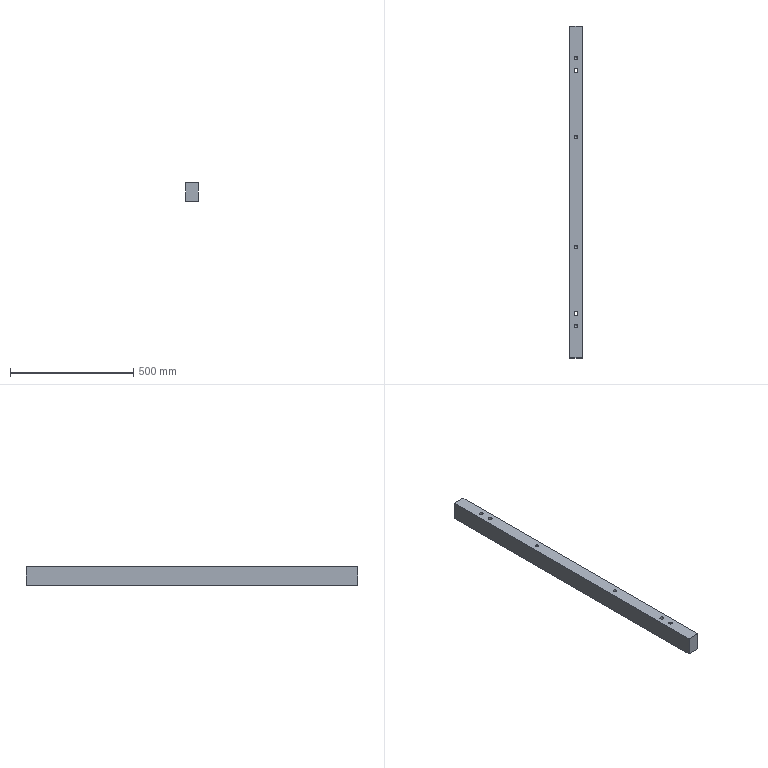Part | NX | features 3 2 | 1 solid | 24 faces | box 50 x 1345 x 75.5 mm | volume 5034144 mm3 | cylinder 10 | cone 8 | plane 6 | commonest cylinder face diameters 14.1 x8 16.001 x2
STEP:
#1=CARTESIAN_POINT('',(-62.95,-542.5,256.5));
#2=VERTEX_POINT('',#1);
#3=CARTESIAN_POINT('',(-70.,-542.5,256.5));
#4=DIRECTION('',(0.,0.,-1.));
#5=DIRECTION('',(1.,0.,0.));
#6=AXIS2_PLACEMENT_3D('',#3,#4,#5);
#7=CIRCLE('',#6,7.05);
#8=EDGE_CURVE('',#2,#2,#7,.T.);
#9=ORIENTED_EDGE('',*,*,#8,.T.);
#10=EDGE_LOOP('',(#9));
#11=FACE_BOUND('',#10,.T.);
#12=CARTESIAN_POINT('',(-62.95,222.5,256.5));
#13=VERTEX_POINT('',#12);
#14=CARTESIAN_POINT('',(-70.,222.5,256.5));
#15=DIRECTION('',(0.,0.,-1.));
#16=DIRECTION('',(1.,0.,0.));
#17=AXIS2_PLACEMENT_3D('',#14,#15,#16);
#18=CIRCLE('',#17,7.05);
#19=EDGE_CURVE('',#13,#13,#18,.T.);
#20=ORIENTED_EDGE('',*,*,#19,.T.);
#21=EDGE_LOOP('',(#20));
#22=FACE_BOUND('',#21,.T.);
#23=CARTESIAN_POINT('',(-45.,-672.5,256.5));
#24=VERTEX_POINT('',#23);
#25=CARTESIAN_POINT('',(-95.,-672.5,256.5));
#26=VERTEX_POINT('',#25);
#27=CARTESIAN_POINT('',(282.5,-672.5,256.5));
#28=DIRECTION('',(-1.,0.,0.));
#29=VECTOR('',#28,1000.);
#30=LINE('',#27,#29);
#31=EDGE_CURVE('',#24,#26,#30,.T.);
#32=ORIENTED_EDGE('',*,*,#31,.F.);
#33=CARTESIAN_POINT('',(-45.,672.5,256.5));
#34=VERTEX_POINT('',#33);
#35=CARTESIAN_POINT('',(-45.,193.,256.5));
#36=DIRECTION('',(0.,-1.,0.));
#37=VECTOR('',#36,1000.);
#38=LINE('',#35,#37);
#39=EDGE_CURVE('',#34,#24,#38,.T.);
#40=ORIENTED_EDGE('',*,*,#39,.F.);
#41=CARTESIAN_POINT('',(-95.,672.5,256.5));
#42=VERTEX_POINT('',#41);
#43=CARTESIAN_POINT('',(-95.,672.5,256.5));
#44=DIRECTION('',(1.,0.,0.));
#45=VECTOR('',#44,1000.);
#46=LINE('',#43,#45);
#47=EDGE_CURVE('',#42,#34,#46,.T.);
#48=ORIENTED_EDGE('',*,*,#47,.F.);
#49=CARTESIAN_POINT('',(-95.,193.,256.5));
#50=DIRECTION('',(0.,1.,0.));
#51=VECTOR('',#50,1000.);
#52=LINE('',#49,#51);
#53=EDGE_CURVE('',#26,#42,#52,.T.);
#54=ORIENTED_EDGE('',*,*,#53,.F.);
#55=EDGE_LOOP('',(#32,#40,#48,#54));
#56=FACE_BOUND('',#55,.T.);
#57=CARTESIAN_POINT('',(-61.999,-492.5,256.5));
#58=VERTEX_POINT('',#57);
#59=CARTESIAN_POINT('',(-70.,-492.5,256.5));
#60=DIRECTION('',(0.,0.,-1.));
#61=DIRECTION('',(1.,0.,0.));
#62=AXIS2_PLACEMENT_3D('',#59,#60,#61);
#63=CIRCLE('',#62,8.001);
#64=EDGE_CURVE('',#58,#58,#63,.T.);
#65=ORIENTED_EDGE('',*,*,#64,.T.);
#66=EDGE_LOOP('',(#65));
#67=FACE_BOUND('',#66,.T.);
#68=CARTESIAN_POINT('',(-61.999,492.5,256.5));
#69=VERTEX_POINT('',#68);
#70=CARTESIAN_POINT('',(-70.,492.5,256.5));
#71=DIRECTION('',(0.,0.,-1.));
#72=DIRECTION('',(1.,0.,0.));
#73=AXIS2_PLACEMENT_3D('',#70,#71,#72);
#74=CIRCLE('',#73,8.001);
#75=EDGE_CURVE('',#69,#69,#74,.T.);
#76=ORIENTED_EDGE('',*,*,#75,.T.);
#77=EDGE_LOOP('',(#76));
#78=FACE_BOUND('',#77,.T.);
#79=CARTESIAN_POINT('',(-62.95,-222.5,256.5));
#80=VERTEX_POINT('',#79);
#81=CARTESIAN_POINT('',(-70.,-222.5,256.5));
#82=DIRECTION('',(0.,0.,-1.));
#83=DIRECTION('',(1.,0.,0.));
#84=AXIS2_PLACEMENT_3D('',#81,#82,#83);
#85=CIRCLE('',#84,7.05);
#86=EDGE_CURVE('',#80,#80,#85,.T.);
#87=ORIENTED_EDGE('',*,*,#86,.T.);
#88=EDGE_LOOP('',(#87));
#89=FACE_BOUND('',#88,.T.);
#90=CARTESIAN_POINT('',(-62.95,542.5,256.5));
#91=VERTEX_POINT('',#90);
#92=CARTESIAN_POINT('',(-70.,542.5,256.5));
#93=DIRECTION('',(0.,0.,-1.));
#94=DIRECTION('',(1.,0.,0.));
#95=AXIS2_PLACEMENT_3D('',#92,#93,#94);
#96=CIRCLE('',#95,7.05);
#97=EDGE_CURVE('',#91,#91,#96,.T.);
#98=ORIENTED_EDGE('',*,*,#97,.T.);
#99=EDGE_LOOP('',(#98));
#100=FACE_BOUND('',#99,.T.);
#101=CARTESIAN_POINT('',(1945.,0.,256.5));
#102=DIRECTION('',(0.,0.,1.));
#103=DIRECTION('',(-1.,0.,0.));
#104=AXIS2_PLACEMENT_3D('',#101,#102,#103);
#105=PLANE('',#104);
#106=ADVANCED_FACE('',(#11,#22,#56,#67,#78,#89,#100),#105,.T.);
#107=CARTESIAN_POINT('',(-62.95,222.5,181.));
#108=VERTEX_POINT('',#107);
#109=CARTESIAN_POINT('',(-70.,222.5,181.));
#110=DIRECTION('',(0.,0.,1.));
#111=DIRECTION('',(1.,0.,0.));
#112=AXIS2_PLACEMENT_3D('',#109,#110,#111);
#113=CIRCLE('',#112,7.05);
#114=EDGE_CURVE('',#108,#108,#113,.T.);
#115=ORIENTED_EDGE('',*,*,#114,.T.);
#116=EDGE_LOOP('',(#115));
#117=FACE_BOUND('',#116,.T.);
#118=CARTESIAN_POINT('',(-62.95,-542.5,181.));
#119=VERTEX_POINT('',#118);
#120=CARTESIAN_POINT('',(-70.,-542.5,181.));
#121=DIRECTION('',(0.,0.,1.));
#122=DIRECTION('',(1.,0.,0.));
#123=AXIS2_PLACEMENT_3D('',#120,#121,#122);
#124=CIRCLE('',#123,7.05);
#125=EDGE_CURVE('',#119,#119,#124,.T.);
#126=ORIENTED_EDGE('',*,*,#125,.T.);
#127=EDGE_LOOP('',(#126));
#128=FACE_BOUND('',#127,.T.);
#129=CARTESIAN_POINT('',(-95.,672.5,181.));
#130=VERTEX_POINT('',#129);
#131=CARTESIAN_POINT('',(-95.,-672.5,181.));
#132=VERTEX_POINT('',#131);
#133=CARTESIAN_POINT('',(-95.,193.,181.));
#134=DIRECTION('',(0.,-1.,0.));
#135=VECTOR('',#134,1000.);
#136=LINE('',#133,#135);
#137=EDGE_CURVE('',#130,#132,#136,.T.);
#138=ORIENTED_EDGE('',*,*,#137,.F.);
#139=CARTESIAN_POINT('',(-45.,672.5,181.));
#140=VERTEX_POINT('',#139);
#141=CARTESIAN_POINT('',(1175.,672.5,181.));
#142=DIRECTION('',(1.,0.,0.));
#143=VECTOR('',#142,1000.);
#144=LINE('',#141,#143);
#145=EDGE_CURVE('',#130,#140,#144,.T.);
#146=ORIENTED_EDGE('',*,*,#145,.T.);
#147=CARTESIAN_POINT('',(-45.,-672.5,181.));
#148=VERTEX_POINT('',#147);
#149=CARTESIAN_POINT('',(-45.,193.,181.));
#150=DIRECTION('',(0.,1.,0.));
#151=VECTOR('',#150,1000.);
#152=LINE('',#149,#151);
#153=EDGE_CURVE('',#148,#140,#152,.T.);
#154=ORIENTED_EDGE('',*,*,#153,.F.);
#155=CARTESIAN_POINT('',(1175.,-672.5,181.));
#156=DIRECTION('',(-1.,0.,0.));
#157=VECTOR('',#156,1000.);
#158=LINE('',#155,#157);
#159=EDGE_CURVE('',#148,#132,#158,.T.);
#160=ORIENTED_EDGE('',*,*,#159,.T.);
#161=EDGE_LOOP('',(#138,#146,#154,#160));
#162=FACE_BOUND('',#161,.T.);
#163=CARTESIAN_POINT('',(-62.95,-222.5,181.));
#164=VERTEX_POINT('',#163);
#165=CARTESIAN_POINT('',(-70.,-222.5,181.));
#166=DIRECTION('',(0.,0.,1.));
#167=DIRECTION('',(1.,0.,0.));
#168=AXIS2_PLACEMENT_3D('',#165,#166,#167);
#169=CIRCLE('',#168,7.05);
#170=EDGE_CURVE('',#164,#164,#169,.T.);
#171=ORIENTED_EDGE('',*,*,#170,.T.);
#172=EDGE_LOOP('',(#171));
#173=FACE_BOUND('',#172,.T.);
#174=CARTESIAN_POINT('',(-62.95,542.5,181.));
#175=VERTEX_POINT('',#174);
#176=CARTESIAN_POINT('',(-70.,542.5,181.));
#177=DIRECTION('',(0.,0.,1.));
#178=DIRECTION('',(1.,0.,0.));
#179=AXIS2_PLACEMENT_3D('',#176,#177,#178);
#180=CIRCLE('',#179,7.05);
#181=EDGE_CURVE('',#175,#175,#180,.T.);
#182=ORIENTED_EDGE('',*,*,#181,.T.);
#183=EDGE_LOOP('',(#182));
#184=FACE_BOUND('',#183,.T.);
#185=CARTESIAN_POINT('',(-78.001,492.5,181.));
#186=VERTEX_POINT('',#185);
#187=CARTESIAN_POINT('',(-70.,492.5,181.));
#188=DIRECTION('',(0.,0.,1.));
#189=DIRECTION('',(-1.,0.,0.));
#190=AXIS2_PLACEMENT_3D('',#187,#188,#189);
#191=CIRCLE('',#190,8.001);
#192=EDGE_CURVE('',#186,#186,#191,.T.);
#193=ORIENTED_EDGE('',*,*,#192,.T.);
#194=EDGE_LOOP('',(#193));
#195=FACE_BOUND('',#194,.T.);
#196=CARTESIAN_POINT('',(-78.001,-492.5,181.));
#197=VERTEX_POINT('',#196);
#198=CARTESIAN_POINT('',(-70.,-492.5,181.));
#199=DIRECTION('',(0.,0.,1.));
#200=DIRECTION('',(-1.,0.,0.));
#201=AXIS2_PLACEMENT_3D('',#198,#199,#200);
#202=CIRCLE('',#201,8.001);
#203=EDGE_CURVE('',#197,#197,#202,.T.);
#204=ORIENTED_EDGE('',*,*,#203,.T.);
#205=EDGE_LOOP('',(#204));
#206=FACE_BOUND('',#205,.T.);
#207=CARTESIAN_POINT('',(1175.,193.,181.));
#208=DIRECTION('',(0.,0.,-1.));
#209=DIRECTION('',(-1.,0.,0.));
#210=AXIS2_PLACEMENT_3D('',#207,#208,#209);
#211=PLANE('',#210);
#212=ADVANCED_FACE('',(#117,#128,#162,#173,#184,#195,#206),#211,.T.);
#213=CARTESIAN_POINT('',(-95.,-672.5,-1.5));
#214=DIRECTION('',(0.,0.,1.));
#215=VECTOR('',#214,1000.);
#216=LINE('',#213,#215);
#217=EDGE_CURVE('',#132,#26,#216,.T.);
#218=ORIENTED_EDGE('',*,*,#217,.T.);
#219=ORIENTED_EDGE('',*,*,#53,.T.);
#220=CARTESIAN_POINT('',(-95.,672.5,-1.5));
#221=DIRECTION('',(0.,0.,-1.));
#222=VECTOR('',#221,1000.);
#223=LINE('',#220,#222);
#224=EDGE_CURVE('',#42,#130,#223,.T.);
#225=ORIENTED_EDGE('',*,*,#224,.T.);
#226=ORIENTED_EDGE('',*,*,#137,.T.);
#227=EDGE_LOOP('',(#218,#219,#225,#226));
#228=FACE_BOUND('',#227,.T.);
#229=CARTESIAN_POINT('',(-95.,193.,-1.5));
#230=DIRECTION('',(-1.,0.,0.));
#231=DIRECTION('',(0.,0.,-1.));
#232=AXIS2_PLACEMENT_3D('',#229,#230,#231);
#233=PLANE('',#232);
#234=ADVANCED_FACE('',(#228),#233,.T.);
#235=CARTESIAN_POINT('',(-45.,672.5,-1.5));
#236=DIRECTION('',(0.,0.,1.));
#237=VECTOR('',#236,1000.);
#238=LINE('',#235,#237);
#239=EDGE_CURVE('',#140,#34,#238,.T.);
#240=ORIENTED_EDGE('',*,*,#239,.T.);
#241=ORIENTED_EDGE('',*,*,#39,.T.);
#242=CARTESIAN_POINT('',(-45.,-672.5,-1.5));
#243=DIRECTION('',(0.,0.,-1.));
#244=VECTOR('',#243,1000.);
#245=LINE('',#242,#244);
#246=EDGE_CURVE('',#24,#148,#245,.T.);
#247=ORIENTED_EDGE('',*,*,#246,.T.);
#248=ORIENTED_EDGE('',*,*,#153,.T.);
#249=EDGE_LOOP('',(#240,#241,#247,#248));
#250=FACE_BOUND('',#249,.T.);
#251=CARTESIAN_POINT('',(-45.,193.,-1.5));
#252=DIRECTION('',(1.,0.,0.));
#253=DIRECTION('',(0.,0.,1.));
#254=AXIS2_PLACEMENT_3D('',#251,#252,#253);
#255=PLANE('',#254);
#256=ADVANCED_FACE('',(#250),#255,.T.);
#257=ORIENTED_EDGE('',*,*,#246,.F.);
#258=ORIENTED_EDGE('',*,*,#31,.T.);
#259=ORIENTED_EDGE('',*,*,#217,.F.);
#260=ORIENTED_EDGE('',*,*,#159,.F.);
#261=EDGE_LOOP('',(#257,#258,#259,#260));
#262=FACE_BOUND('',#261,.T.);
#263=CARTESIAN_POINT('',(282.5,-672.5,-103.));
#264=DIRECTION('',(0.,1.,0.));
#265=DIRECTION('',(1.,0.,0.));
#266=AXIS2_PLACEMENT_3D('',#263,#264,#265);
#267=PLANE('',#266);
#268=ADVANCED_FACE('',(#262),#267,.F.);
#269=ORIENTED_EDGE('',*,*,#224,.F.);
#270=ORIENTED_EDGE('',*,*,#47,.T.);
#271=ORIENTED_EDGE('',*,*,#239,.F.);
#272=ORIENTED_EDGE('',*,*,#145,.F.);
#273=EDGE_LOOP('',(#269,#270,#271,#272));
#274=FACE_BOUND('',#273,.T.);
#275=CARTESIAN_POINT('',(-95.,672.5,231.5));
#276=DIRECTION('',(0.,1.,0.));
#277=DIRECTION('',(0.,0.,-1.));
#278=AXIS2_PLACEMENT_3D('',#275,#276,#277);
#279=PLANE('',#278);
#280=ADVANCED_FACE('',(#274),#279,.T.);
#281=ORIENTED_EDGE('',*,*,#125,.F.);
#282=EDGE_LOOP('',(#281));
#283=FACE_BOUND('',#282,.T.);
#284=CARTESIAN_POINT('',(-62.95,-542.5,188.95));
#285=VERTEX_POINT('',#284);
#286=CARTESIAN_POINT('',(-70.,-542.5,188.95));
#287=DIRECTION('',(0.,0.,-1.));
#288=DIRECTION('',(1.,0.,0.));
#289=AXIS2_PLACEMENT_3D('',#286,#287,#288);
#290=CIRCLE('',#289,7.05);
#291=EDGE_CURVE('',#285,#285,#290,.T.);
#292=ORIENTED_EDGE('',*,*,#291,.F.);
#293=EDGE_LOOP('',(#292));
#294=FACE_BOUND('',#293,.T.);
#295=CARTESIAN_POINT('',(-70.,-542.5,181.));
#296=DIRECTION('',(0.,0.,1.));
#297=DIRECTION('',(-1.,0.,0.));
#298=AXIS2_PLACEMENT_3D('',#295,#296,#297);
#299=CYLINDRICAL_SURFACE('',#298,7.05);
#300=ADVANCED_FACE('',(#283,#294),#299,.F.);
#301=ORIENTED_EDGE('',*,*,#170,.F.);
#302=EDGE_LOOP('',(#301));
#303=FACE_BOUND('',#302,.T.);
#304=CARTESIAN_POINT('',(-62.95,-222.5,188.95));
#305=VERTEX_POINT('',#304);
#306=CARTESIAN_POINT('',(-70.,-222.5,188.95));
#307=DIRECTION('',(0.,0.,-1.));
#308=DIRECTION('',(1.,0.,0.));
#309=AXIS2_PLACEMENT_3D('',#306,#307,#308);
#310=CIRCLE('',#309,7.05);
#311=EDGE_CURVE('',#305,#305,#310,.T.);
#312=ORIENTED_EDGE('',*,*,#311,.F.);
#313=EDGE_LOOP('',(#312));
#314=FACE_BOUND('',#313,.T.);
#315=CARTESIAN_POINT('',(-70.,-222.5,181.));
#316=DIRECTION('',(0.,0.,1.));
#317=DIRECTION('',(-1.,0.,0.));
#318=AXIS2_PLACEMENT_3D('',#315,#316,#317);
#319=CYLINDRICAL_SURFACE('',#318,7.05);
#320=ADVANCED_FACE('',(#303,#314),#319,.F.);
#321=ORIENTED_EDGE('',*,*,#114,.F.);
#322=EDGE_LOOP('',(#321));
#323=FACE_BOUND('',#322,.T.);
#324=CARTESIAN_POINT('',(-62.95,222.5,188.95));
#325=VERTEX_POINT('',#324);
#326=CARTESIAN_POINT('',(-70.,222.5,188.95));
#327=DIRECTION('',(0.,0.,-1.));
#328=DIRECTION('',(1.,0.,0.));
#329=AXIS2_PLACEMENT_3D('',#326,#327,#328);
#330=CIRCLE('',#329,7.05);
#331=EDGE_CURVE('',#325,#325,#330,.T.);
#332=ORIENTED_EDGE('',*,*,#331,.F.);
#333=EDGE_LOOP('',(#332));
#334=FACE_BOUND('',#333,.T.);
#335=CARTESIAN_POINT('',(-70.,222.5,181.));
#336=DIRECTION('',(0.,0.,1.));
#337=DIRECTION('',(-1.,0.,0.));
#338=AXIS2_PLACEMENT_3D('',#335,#336,#337);
#339=CYLINDRICAL_SURFACE('',#338,7.05);
#340=ADVANCED_FACE('',(#323,#334),#339,.F.);
#341=ORIENTED_EDGE('',*,*,#181,.F.);
#342=EDGE_LOOP('',(#341));
#343=FACE_BOUND('',#342,.T.);
#344=CARTESIAN_POINT('',(-62.95,542.5,188.95));
#345=VERTEX_POINT('',#344);
#346=CARTESIAN_POINT('',(-70.,542.5,188.95));
#347=DIRECTION('',(0.,0.,-1.));
#348=DIRECTION('',(1.,0.,0.));
#349=AXIS2_PLACEMENT_3D('',#346,#347,#348);
#350=CIRCLE('',#349,7.05);
#351=EDGE_CURVE('',#345,#345,#350,.T.);
#352=ORIENTED_EDGE('',*,*,#351,.F.);
#353=EDGE_LOOP('',(#352));
#354=FACE_BOUND('',#353,.T.);
#355=CARTESIAN_POINT('',(-70.,542.5,181.));
#356=DIRECTION('',(0.,0.,1.));
#357=DIRECTION('',(-1.,0.,0.));
#358=AXIS2_PLACEMENT_3D('',#355,#356,#357);
#359=CYLINDRICAL_SURFACE('',#358,7.05);
#360=ADVANCED_FACE('',(#343,#354),#359,.F.);
#361=ORIENTED_EDGE('',*,*,#192,.F.);
#362=EDGE_LOOP('',(#361));
#363=FACE_BOUND('',#362,.T.);
#364=ORIENTED_EDGE('',*,*,#75,.F.);
#365=EDGE_LOOP('',(#364));
#366=FACE_BOUND('',#365,.T.);
#367=CARTESIAN_POINT('',(-70.,492.5,181.));
#368=DIRECTION('',(0.,0.,1.));
#369=DIRECTION('',(-1.,0.,0.));
#370=AXIS2_PLACEMENT_3D('',#367,#368,#369);
#371=CYLINDRICAL_SURFACE('',#370,8.001);
#372=ADVANCED_FACE('',(#363,#366),#371,.F.);
#373=ORIENTED_EDGE('',*,*,#203,.F.);
#374=EDGE_LOOP('',(#373));
#375=FACE_BOUND('',#374,.T.);
#376=ORIENTED_EDGE('',*,*,#64,.F.);
#377=EDGE_LOOP('',(#376));
#378=FACE_BOUND('',#377,.T.);
#379=CARTESIAN_POINT('',(-70.,-492.5,181.));
#380=DIRECTION('',(0.,0.,1.));
#381=DIRECTION('',(-1.,0.,0.));
#382=AXIS2_PLACEMENT_3D('',#379,#380,#381);
#383=CYLINDRICAL_SURFACE('',#382,8.001);
#384=ADVANCED_FACE('',(#375,#378),#383,.F.);
#385=CARTESIAN_POINT('',(-70.,-542.5,196.));
#386=VERTEX_POINT('',#385);
#387=VERTEX_LOOP('',#386);
#388=FACE_BOUND('',#387,.T.);
#389=ORIENTED_EDGE('',*,*,#291,.T.);
#390=EDGE_LOOP('',(#389));
#391=FACE_BOUND('',#390,.T.);
#392=CARTESIAN_POINT('',(-70.,-542.5,188.95));
#393=DIRECTION('',(0.,0.,-1.));
#394=DIRECTION('',(1.,0.,0.));
#395=AXIS2_PLACEMENT_3D('',#392,#393,#394);
#396=CONICAL_SURFACE('',#395,7.05,0.7854);
#397=ADVANCED_FACE('',(#388,#391),#396,.F.);
#398=CARTESIAN_POINT('',(-70.,-222.5,196.));
#399=VERTEX_POINT('',#398);
#400=VERTEX_LOOP('',#399);
#401=FACE_BOUND('',#400,.T.);
#402=ORIENTED_EDGE('',*,*,#311,.T.);
#403=EDGE_LOOP('',(#402));
#404=FACE_BOUND('',#403,.T.);
#405=CARTESIAN_POINT('',(-70.,-222.5,188.95));
#406=DIRECTION('',(0.,0.,-1.));
#407=DIRECTION('',(1.,0.,0.));
#408=AXIS2_PLACEMENT_3D('',#405,#406,#407);
#409=CONICAL_SURFACE('',#408,7.05,0.7854);
#410=ADVANCED_FACE('',(#401,#404),#409,.F.);
#411=CARTESIAN_POINT('',(-70.,222.5,196.));
#412=VERTEX_POINT('',#411);
#413=VERTEX_LOOP('',#412);
#414=FACE_BOUND('',#413,.T.);
#415=ORIENTED_EDGE('',*,*,#331,.T.);
#416=EDGE_LOOP('',(#415));
#417=FACE_BOUND('',#416,.T.);
#418=CARTESIAN_POINT('',(-70.,222.5,188.95));
#419=DIRECTION('',(0.,0.,-1.));
#420=DIRECTION('',(1.,0.,0.));
#421=AXIS2_PLACEMENT_3D('',#418,#419,#420);
#422=CONICAL_SURFACE('',#421,7.05,0.7854);
#423=ADVANCED_FACE('',(#414,#417),#422,.F.);
#424=CARTESIAN_POINT('',(-70.,542.5,196.));
#425=VERTEX_POINT('',#424);
#426=VERTEX_LOOP('',#425);
#427=FACE_BOUND('',#426,.T.);
#428=ORIENTED_EDGE('',*,*,#351,.T.);
#429=EDGE_LOOP('',(#428));
#430=FACE_BOUND('',#429,.T.);
#431=CARTESIAN_POINT('',(-70.,542.5,188.95));
#432=DIRECTION('',(0.,0.,-1.));
#433=DIRECTION('',(1.,0.,0.));
#434=AXIS2_PLACEMENT_3D('',#431,#432,#433);
#435=CONICAL_SURFACE('',#434,7.05,0.7854);
#436=ADVANCED_FACE('',(#427,#430),#435,.F.);
#437=CARTESIAN_POINT('',(-77.05,222.5,248.55));
#438=VERTEX_POINT('',#437);
#439=CARTESIAN_POINT('',(-70.,222.5,248.55));
#440=DIRECTION('',(0.,0.,-1.));
#441=DIRECTION('',(-1.,0.,0.));
#442=AXIS2_PLACEMENT_3D('',#439,#440,#441);
#443=CIRCLE('',#442,7.05);
#444=EDGE_CURVE('',#438,#438,#443,.T.);
#445=ORIENTED_EDGE('',*,*,#444,.T.);
#446=EDGE_LOOP('',(#445));
#447=FACE_BOUND('',#446,.T.);
#448=ORIENTED_EDGE('',*,*,#19,.F.);
#449=EDGE_LOOP('',(#448));
#450=FACE_BOUND('',#449,.T.);
#451=CARTESIAN_POINT('',(-70.,222.5,256.5));
#452=DIRECTION('',(0.,0.,-1.));
#453=DIRECTION('',(-1.,0.,0.));
#454=AXIS2_PLACEMENT_3D('',#451,#452,#453);
#455=CYLINDRICAL_SURFACE('',#454,7.05);
#456=ADVANCED_FACE('',(#447,#450),#455,.F.);
#457=CARTESIAN_POINT('',(-70.,222.5,241.5));
#458=VERTEX_POINT('',#457);
#459=VERTEX_LOOP('',#458);
#460=FACE_BOUND('',#459,.T.);
#461=ORIENTED_EDGE('',*,*,#444,.F.);
#462=EDGE_LOOP('',(#461));
#463=FACE_BOUND('',#462,.T.);
#464=CARTESIAN_POINT('',(-70.,222.5,248.55));
#465=DIRECTION('',(0.,0.,1.));
#466=DIRECTION('',(-1.,0.,0.));
#467=AXIS2_PLACEMENT_3D('',#464,#465,#466);
#468=CONICAL_SURFACE('',#467,7.05,0.7854);
#469=ADVANCED_FACE('',(#460,#463),#468,.F.);
#470=CARTESIAN_POINT('',(-77.05,-222.5,248.55));
#471=VERTEX_POINT('',#470);
#472=CARTESIAN_POINT('',(-70.,-222.5,248.55));
#473=DIRECTION('',(0.,0.,-1.));
#474=DIRECTION('',(-1.,0.,0.));
#475=AXIS2_PLACEMENT_3D('',#472,#473,#474);
#476=CIRCLE('',#475,7.05);
#477=EDGE_CURVE('',#471,#471,#476,.T.);
#478=ORIENTED_EDGE('',*,*,#477,.T.);
#479=EDGE_LOOP('',(#478));
#480=FACE_BOUND('',#479,.T.);
#481=ORIENTED_EDGE('',*,*,#86,.F.);
#482=EDGE_LOOP('',(#481));
#483=FACE_BOUND('',#482,.T.);
#484=CARTESIAN_POINT('',(-70.,-222.5,256.5));
#485=DIRECTION('',(0.,0.,-1.));
#486=DIRECTION('',(-1.,0.,0.));
#487=AXIS2_PLACEMENT_3D('',#484,#485,#486);
#488=CYLINDRICAL_SURFACE('',#487,7.05);
#489=ADVANCED_FACE('',(#480,#483),#488,.F.);
#490=CARTESIAN_POINT('',(-70.,-222.5,241.5));
#491=VERTEX_POINT('',#490);
#492=VERTEX_LOOP('',#491);
#493=FACE_BOUND('',#492,.T.);
#494=ORIENTED_EDGE('',*,*,#477,.F.);
#495=EDGE_LOOP('',(#494));
#496=FACE_BOUND('',#495,.T.);
#497=CARTESIAN_POINT('',(-70.,-222.5,248.55));
#498=DIRECTION('',(0.,0.,1.));
#499=DIRECTION('',(-1.,0.,0.));
#500=AXIS2_PLACEMENT_3D('',#497,#498,#499);
#501=CONICAL_SURFACE('',#500,7.05,0.7854);
#502=ADVANCED_FACE('',(#493,#496),#501,.F.);
#503=CARTESIAN_POINT('',(-77.05,-542.5,248.55));
#504=VERTEX_POINT('',#503);
#505=CARTESIAN_POINT('',(-70.,-542.5,248.55));
#506=DIRECTION('',(0.,0.,-1.));
#507=DIRECTION('',(-1.,0.,0.));
#508=AXIS2_PLACEMENT_3D('',#505,#506,#507);
#509=CIRCLE('',#508,7.05);
#510=EDGE_CURVE('',#504,#504,#509,.T.);
#511=ORIENTED_EDGE('',*,*,#510,.T.);
#512=EDGE_LOOP('',(#511));
#513=FACE_BOUND('',#512,.T.);
#514=ORIENTED_EDGE('',*,*,#8,.F.);
#515=EDGE_LOOP('',(#514));
#516=FACE_BOUND('',#515,.T.);
#517=CARTESIAN_POINT('',(-70.,-542.5,256.5));
#518=DIRECTION('',(0.,0.,-1.));
#519=DIRECTION('',(-1.,0.,0.));
#520=AXIS2_PLACEMENT_3D('',#517,#518,#519);
#521=CYLINDRICAL_SURFACE('',#520,7.05);
#522=ADVANCED_FACE('',(#513,#516),#521,.F.);
#523=CARTESIAN_POINT('',(-70.,-542.5,241.5));
#524=VERTEX_POINT('',#523);
#525=VERTEX_LOOP('',#524);
#526=FACE_BOUND('',#525,.T.);
#527=ORIENTED_EDGE('',*,*,#510,.F.);
#528=EDGE_LOOP('',(#527));
#529=FACE_BOUND('',#528,.T.);
#530=CARTESIAN_POINT('',(-70.,-542.5,248.55));
#531=DIRECTION('',(0.,0.,1.));
#532=DIRECTION('',(-1.,0.,0.));
#533=AXIS2_PLACEMENT_3D('',#530,#531,#532);
#534=CONICAL_SURFACE('',#533,7.05,0.7854);
#535=ADVANCED_FACE('',(#526,#529),#534,.F.);
#536=CARTESIAN_POINT('',(-77.05,542.5,248.55));
#537=VERTEX_POINT('',#536);
#538=CARTESIAN_POINT('',(-70.,542.5,248.55));
#539=DIRECTION('',(0.,0.,-1.));
#540=DIRECTION('',(-1.,0.,0.));
#541=AXIS2_PLACEMENT_3D('',#538,#539,#540);
#542=CIRCLE('',#541,7.05);
#543=EDGE_CURVE('',#537,#537,#542,.T.);
#544=ORIENTED_EDGE('',*,*,#543,.T.);
#545=EDGE_LOOP('',(#544));
#546=FACE_BOUND('',#545,.T.);
#547=ORIENTED_EDGE('',*,*,#97,.F.);
#548=EDGE_LOOP('',(#547));
#549=FACE_BOUND('',#548,.T.);
#550=CARTESIAN_POINT('',(-70.,542.5,256.5));
#551=DIRECTION('',(0.,0.,-1.));
#552=DIRECTION('',(-1.,0.,0.));
#553=AXIS2_PLACEMENT_3D('',#550,#551,#552);
#554=CYLINDRICAL_SURFACE('',#553,7.05);
#555=ADVANCED_FACE('',(#546,#549),#554,.F.);
#556=CARTESIAN_POINT('',(-70.,542.5,241.5));
#557=VERTEX_POINT('',#556);
#558=VERTEX_LOOP('',#557);
#559=FACE_BOUND('',#558,.T.);
#560=ORIENTED_EDGE('',*,*,#543,.F.);
#561=EDGE_LOOP('',(#560));
#562=FACE_BOUND('',#561,.T.);
#563=CARTESIAN_POINT('',(-70.,542.5,248.55));
#564=DIRECTION('',(0.,0.,1.));
#565=DIRECTION('',(-1.,0.,0.));
#566=AXIS2_PLACEMENT_3D('',#563,#564,#565);
#567=CONICAL_SURFACE('',#566,7.05,0.7854);
#568=ADVANCED_FACE('',(#559,#562),#567,.F.);
#569=CLOSED_SHELL('',(#106,#212,#234,#256,#268,#280,#300,#320,#340,#360,#372,#384,#397,#410,#423,#436,#456,#469,#489,#502,#522,#535,#555,#568));
#570=MANIFOLD_SOLID_BREP('',#569);
#571=(LENGTH_UNIT()NAMED_UNIT(*)SI_UNIT(.MILLI.,.METRE.));
#572=UNCERTAINTY_MEASURE_WITH_UNIT(LENGTH_MEASURE(0.00001),#571,'','');
#573=(NAMED_UNIT(*)PLANE_ANGLE_UNIT()SI_UNIT($,.RADIAN.));
#574=(NAMED_UNIT(*)SI_UNIT($,.STERADIAN.)SOLID_ANGLE_UNIT());
#575=(GEOMETRIC_REPRESENTATION_CONTEXT(3)GLOBAL_UNCERTAINTY_ASSIGNED_CONTEXT((#572))GLOBAL_UNIT_ASSIGNED_CONTEXT((#571,#573,#574))REPRESENTATION_CONTEXT('',''));
#576=ADVANCED_BREP_SHAPE_REPRESENTATION('',(#570),#575);